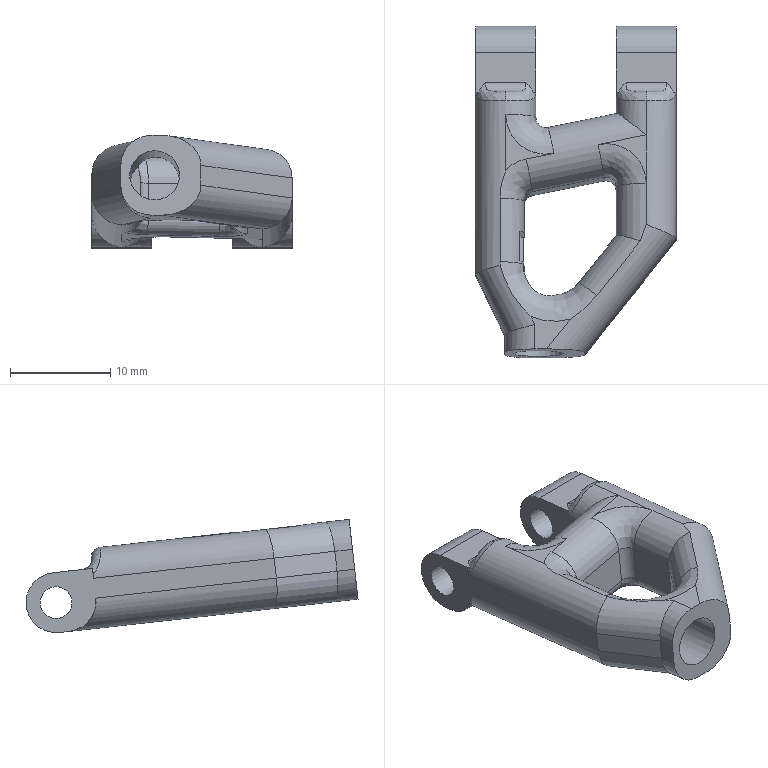Part | STEP file | Wytnij-wyci_gni_cie2 | 1 solid | 79 faces | box 20 x 33.148 x 11.306 mm | volume 2601 mm3 | cylinder 37 | plane 28 | spline 14 | commonest cylinder face diameters 6 x24 2 x5 3 x4 3.18 x2 4.96 x1 6.4 x1